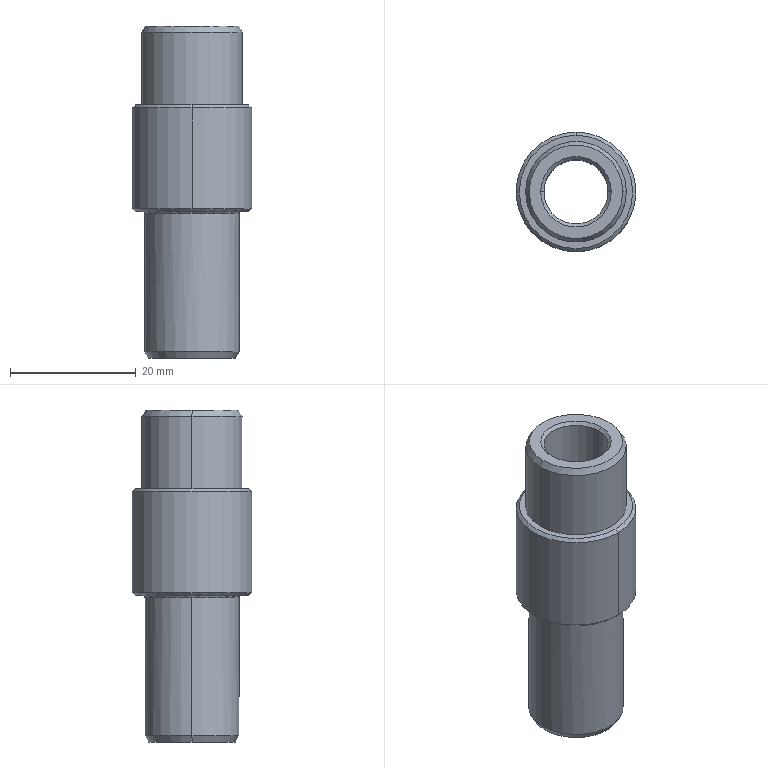Part | STEP file | PERNO RODAJA SUPERIOR | 1 solid | 26 faces | box 19 x 19 x 52.7 mm | volume 7077 mm3 | cone 12 | cylinder 8 | plane 4 | torus 2 | commonest cylinder face diameters 10.2 x2 15 x2 16 x2 19 x2
STEP:
#1=CARTESIAN_POINT('',(7.423,0.,10.5));
#2=VERTEX_POINT('',#1);
#3=CARTESIAN_POINT('',(-7.423,0.,10.5));
#4=VERTEX_POINT('',#3);
#5=CARTESIAN_POINT('',(0.,0.,10.5));
#6=DIRECTION('',(0.,0.,1.));
#7=DIRECTION('',(1.,0.,0.));
#8=AXIS2_PLACEMENT_3D('',#5,#6,#7);
#9=CIRCLE('',#8,7.423);
#10=EDGE_CURVE('',#2,#4,#9,.T.);
#11=ORIENTED_EDGE('',*,*,#10,.F.);
#12=CARTESIAN_POINT('',(8.,0.,9.5));
#13=VERTEX_POINT('',#12);
#14=CARTESIAN_POINT('',(7.423,0.,10.5));
#15=DIRECTION('',(0.5,0.,-0.866));
#16=VECTOR('',#15,1000.);
#17=LINE('',#14,#16);
#18=EDGE_CURVE('',#2,#13,#17,.T.);
#19=ORIENTED_EDGE('',*,*,#18,.T.);
#20=CARTESIAN_POINT('',(-8.,0.,9.5));
#21=VERTEX_POINT('',#20);
#22=CARTESIAN_POINT('',(0.,0.,9.5));
#23=DIRECTION('',(0.,0.,-1.));
#24=DIRECTION('',(1.,0.,0.));
#25=AXIS2_PLACEMENT_3D('',#22,#23,#24);
#26=CIRCLE('',#25,8.);
#27=EDGE_CURVE('',#21,#13,#26,.T.);
#28=ORIENTED_EDGE('',*,*,#27,.F.);
#29=CARTESIAN_POINT('',(-7.423,0.,10.5));
#30=DIRECTION('',(-0.5,0.,-0.866));
#31=VECTOR('',#30,1000.);
#32=LINE('',#29,#31);
#33=EDGE_CURVE('',#4,#21,#32,.T.);
#34=ORIENTED_EDGE('',*,*,#33,.F.);
#35=EDGE_LOOP('',(#11,#19,#28,#34));
#36=FACE_OUTER_BOUND('',#35,.T.);
#37=CARTESIAN_POINT('',(0.,0.,10.5));
#38=DIRECTION('',(0.,0.,-1.));
#39=DIRECTION('',(-1.,0.,0.));
#40=AXIS2_PLACEMENT_3D('',#37,#38,#39);
#41=CONICAL_SURFACE('',#40,7.423,0.5236);
#42=ADVANCED_FACE('',(#36),#41,.T.);
#43=CARTESIAN_POINT('',(0.,-9.,-2.));
#44=VERTEX_POINT('',#43);
#45=CARTESIAN_POINT('',(0.,9.,-2.));
#46=VERTEX_POINT('',#45);
#47=CARTESIAN_POINT('',(0.,0.,-2.));
#48=DIRECTION('',(0.,0.,1.));
#49=DIRECTION('',(0.,-1.,0.));
#50=AXIS2_PLACEMENT_3D('',#47,#48,#49);
#51=CIRCLE('',#50,9.);
#52=EDGE_CURVE('',#44,#46,#51,.T.);
#53=ORIENTED_EDGE('',*,*,#52,.F.);
#54=CARTESIAN_POINT('',(0.,-9.5,-2.5));
#55=VERTEX_POINT('',#54);
#56=CARTESIAN_POINT('',(0.,-9.5,-2.5));
#57=DIRECTION('',(0.,-0.7071,-0.7071));
#58=VECTOR('',#57,1000.);
#59=LINE('',#56,#58);
#60=EDGE_CURVE('',#44,#55,#59,.T.);
#61=ORIENTED_EDGE('',*,*,#60,.T.);
#62=CARTESIAN_POINT('',(0.,9.5,-2.5));
#63=VERTEX_POINT('',#62);
#64=CARTESIAN_POINT('',(0.,0.,-2.5));
#65=DIRECTION('',(0.,0.,-1.));
#66=DIRECTION('',(0.,-1.,0.));
#67=AXIS2_PLACEMENT_3D('',#64,#65,#66);
#68=CIRCLE('',#67,9.5);
#69=EDGE_CURVE('',#63,#55,#68,.T.);
#70=ORIENTED_EDGE('',*,*,#69,.F.);
#71=CARTESIAN_POINT('',(0.,9.5,-2.5));
#72=DIRECTION('',(0.,0.7071,-0.7071));
#73=VECTOR('',#72,1000.);
#74=LINE('',#71,#73);
#75=EDGE_CURVE('',#46,#63,#74,.T.);
#76=ORIENTED_EDGE('',*,*,#75,.F.);
#77=EDGE_LOOP('',(#53,#61,#70,#76));
#78=FACE_OUTER_BOUND('',#77,.T.);
#79=CARTESIAN_POINT('',(0.,0.,-2.5));
#80=DIRECTION('',(0.,0.,-1.));
#81=DIRECTION('',(0.,1.,0.));
#82=AXIS2_PLACEMENT_3D('',#79,#80,#81);
#83=CONICAL_SURFACE('',#82,9.5,0.7854);
#84=ADVANCED_FACE('',(#78),#83,.T.);
#85=CARTESIAN_POINT('',(0.,9.,-19.));
#86=VERTEX_POINT('',#85);
#87=CARTESIAN_POINT('',(0.,-9.,-19.));
#88=VERTEX_POINT('',#87);
#89=CARTESIAN_POINT('',(0.,0.,-19.));
#90=DIRECTION('',(0.,0.,-1.));
#91=DIRECTION('',(0.,1.,0.));
#92=AXIS2_PLACEMENT_3D('',#89,#90,#91);
#93=CIRCLE('',#92,9.);
#94=EDGE_CURVE('',#86,#88,#93,.T.);
#95=ORIENTED_EDGE('',*,*,#94,.F.);
#96=CARTESIAN_POINT('',(0.,9.5,-18.5));
#97=VERTEX_POINT('',#96);
#98=CARTESIAN_POINT('',(0.,9.,-19.));
#99=DIRECTION('',(0.,0.7071,0.7071));
#100=VECTOR('',#99,1000.);
#101=LINE('',#98,#100);
#102=EDGE_CURVE('',#86,#97,#101,.T.);
#103=ORIENTED_EDGE('',*,*,#102,.T.);
#104=CARTESIAN_POINT('',(0.,-9.5,-18.5));
#105=VERTEX_POINT('',#104);
#106=CARTESIAN_POINT('',(0.,0.,-18.5));
#107=DIRECTION('',(0.,0.,1.));
#108=DIRECTION('',(0.,1.,0.));
#109=AXIS2_PLACEMENT_3D('',#106,#107,#108);
#110=CIRCLE('',#109,9.5);
#111=EDGE_CURVE('',#105,#97,#110,.T.);
#112=ORIENTED_EDGE('',*,*,#111,.F.);
#113=CARTESIAN_POINT('',(0.,-9.,-19.));
#114=DIRECTION('',(0.,-0.7071,0.7071));
#115=VECTOR('',#114,1000.);
#116=LINE('',#113,#115);
#117=EDGE_CURVE('',#88,#105,#116,.T.);
#118=ORIENTED_EDGE('',*,*,#117,.F.);
#119=EDGE_LOOP('',(#95,#103,#112,#118));
#120=FACE_OUTER_BOUND('',#119,.T.);
#121=CARTESIAN_POINT('',(0.,0.,-19.));
#122=DIRECTION('',(0.,0.,1.));
#123=DIRECTION('',(0.,-1.,0.));
#124=AXIS2_PLACEMENT_3D('',#121,#122,#123);
#125=CONICAL_SURFACE('',#124,9.,0.7854);
#126=ADVANCED_FACE('',(#120),#125,.T.);
#127=CARTESIAN_POINT('',(-5.1,0.,10.));
#128=VERTEX_POINT('',#127);
#129=CARTESIAN_POINT('',(5.1,0.,10.));
#130=VERTEX_POINT('',#129);
#131=CARTESIAN_POINT('',(0.,0.,10.));
#132=DIRECTION('',(0.,0.,1.));
#133=DIRECTION('',(1.,0.,0.));
#134=AXIS2_PLACEMENT_3D('',#131,#132,#133);
#135=CIRCLE('',#134,5.1);
#136=EDGE_CURVE('',#128,#130,#135,.T.);
#137=ORIENTED_EDGE('',*,*,#136,.F.);
#138=CARTESIAN_POINT('',(-5.6,0.,10.5));
#139=VERTEX_POINT('',#138);
#140=CARTESIAN_POINT('',(-5.6,0.,10.5));
#141=DIRECTION('',(-0.7071,0.,0.7071));
#142=VECTOR('',#141,1000.);
#143=LINE('',#140,#142);
#144=EDGE_CURVE('',#128,#139,#143,.T.);
#145=ORIENTED_EDGE('',*,*,#144,.T.);
#146=CARTESIAN_POINT('',(5.6,0.,10.5));
#147=VERTEX_POINT('',#146);
#148=CARTESIAN_POINT('',(0.,0.,10.5));
#149=DIRECTION('',(0.,0.,-1.));
#150=DIRECTION('',(1.,0.,0.));
#151=AXIS2_PLACEMENT_3D('',#148,#149,#150);
#152=CIRCLE('',#151,5.6);
#153=EDGE_CURVE('',#147,#139,#152,.T.);
#154=ORIENTED_EDGE('',*,*,#153,.F.);
#155=CARTESIAN_POINT('',(5.6,0.,10.5));
#156=DIRECTION('',(0.7071,0.,0.7071));
#157=VECTOR('',#156,1000.);
#158=LINE('',#155,#157);
#159=EDGE_CURVE('',#130,#147,#158,.T.);
#160=ORIENTED_EDGE('',*,*,#159,.F.);
#161=EDGE_LOOP('',(#137,#145,#154,#160));
#162=FACE_OUTER_BOUND('',#161,.T.);
#163=CARTESIAN_POINT('',(0.,0.,10.5));
#164=DIRECTION('',(0.,0.,1.));
#165=DIRECTION('',(1.,0.,0.));
#166=AXIS2_PLACEMENT_3D('',#163,#164,#165);
#167=CONICAL_SURFACE('',#166,5.6,0.7854);
#168=ADVANCED_FACE('',(#162),#167,.F.);
#169=CARTESIAN_POINT('',(5.1,0.,-41.7));
#170=VERTEX_POINT('',#169);
#171=CARTESIAN_POINT('',(-5.1,0.,-41.7));
#172=VERTEX_POINT('',#171);
#173=CARTESIAN_POINT('',(0.,0.,-41.7));
#174=DIRECTION('',(0.,0.,-1.));
#175=DIRECTION('',(1.,0.,0.));
#176=AXIS2_PLACEMENT_3D('',#173,#174,#175);
#177=CIRCLE('',#176,5.1);
#178=EDGE_CURVE('',#170,#172,#177,.T.);
#179=ORIENTED_EDGE('',*,*,#178,.F.);
#180=CARTESIAN_POINT('',(5.6,0.,-42.2));
#181=VERTEX_POINT('',#180);
#182=CARTESIAN_POINT('',(5.1,0.,-41.7));
#183=DIRECTION('',(0.7071,0.,-0.7071));
#184=VECTOR('',#183,1000.);
#185=LINE('',#182,#184);
#186=EDGE_CURVE('',#170,#181,#185,.T.);
#187=ORIENTED_EDGE('',*,*,#186,.T.);
#188=CARTESIAN_POINT('',(-5.6,0.,-42.2));
#189=VERTEX_POINT('',#188);
#190=CARTESIAN_POINT('',(0.,0.,-42.2));
#191=DIRECTION('',(0.,0.,1.));
#192=DIRECTION('',(1.,0.,0.));
#193=AXIS2_PLACEMENT_3D('',#190,#191,#192);
#194=CIRCLE('',#193,5.6);
#195=EDGE_CURVE('',#189,#181,#194,.T.);
#196=ORIENTED_EDGE('',*,*,#195,.F.);
#197=CARTESIAN_POINT('',(-5.1,0.,-41.7));
#198=DIRECTION('',(-0.7071,0.,-0.7071));
#199=VECTOR('',#198,1000.);
#200=LINE('',#197,#199);
#201=EDGE_CURVE('',#172,#189,#200,.T.);
#202=ORIENTED_EDGE('',*,*,#201,.F.);
#203=EDGE_LOOP('',(#179,#187,#196,#202));
#204=FACE_OUTER_BOUND('',#203,.T.);
#205=CARTESIAN_POINT('',(0.,0.,-41.7));
#206=DIRECTION('',(0.,0.,-1.));
#207=DIRECTION('',(-1.,0.,0.));
#208=AXIS2_PLACEMENT_3D('',#205,#206,#207);
#209=CONICAL_SURFACE('',#208,5.1,0.7854);
#210=ADVANCED_FACE('',(#204),#209,.F.);
#211=ORIENTED_EDGE('',*,*,#136,.T.);
#212=CARTESIAN_POINT('',(5.1,0.,-42.2));
#213=DIRECTION('',(0.,0.,-1.));
#214=VECTOR('',#213,1000.);
#215=LINE('',#212,#214);
#216=EDGE_CURVE('',#130,#170,#215,.T.);
#217=ORIENTED_EDGE('',*,*,#216,.T.);
#218=ORIENTED_EDGE('',*,*,#178,.T.);
#219=CARTESIAN_POINT('',(-5.1,0.,-42.2));
#220=DIRECTION('',(0.,0.,-1.));
#221=VECTOR('',#220,1000.);
#222=LINE('',#219,#221);
#223=EDGE_CURVE('',#128,#172,#222,.T.);
#224=ORIENTED_EDGE('',*,*,#223,.F.);
#225=EDGE_LOOP('',(#211,#217,#218,#224));
#226=FACE_OUTER_BOUND('',#225,.T.);
#227=CARTESIAN_POINT('',(0.,0.,-42.2));
#228=DIRECTION('',(0.,0.,-1.));
#229=DIRECTION('',(-1.,0.,0.));
#230=AXIS2_PLACEMENT_3D('',#227,#228,#229);
#231=CYLINDRICAL_SURFACE('',#230,5.1);
#232=ADVANCED_FACE('',(#226),#231,.F.);
#233=CARTESIAN_POINT('',(-6.923,0.,-42.2));
#234=VERTEX_POINT('',#233);
#235=CARTESIAN_POINT('',(6.923,0.,-42.2));
#236=VERTEX_POINT('',#235);
#237=CARTESIAN_POINT('',(0.,0.,-42.2));
#238=DIRECTION('',(0.,0.,-1.));
#239=DIRECTION('',(1.,0.,0.));
#240=AXIS2_PLACEMENT_3D('',#237,#238,#239);
#241=CIRCLE('',#240,6.923);
#242=EDGE_CURVE('',#234,#236,#241,.T.);
#243=ORIENTED_EDGE('',*,*,#242,.F.);
#244=CARTESIAN_POINT('',(-7.5,0.,-41.2));
#245=VERTEX_POINT('',#244);
#246=CARTESIAN_POINT('',(-7.5,0.,-41.2));
#247=DIRECTION('',(-0.5,0.,0.866));
#248=VECTOR('',#247,1000.);
#249=LINE('',#246,#248);
#250=EDGE_CURVE('',#234,#245,#249,.T.);
#251=ORIENTED_EDGE('',*,*,#250,.T.);
#252=CARTESIAN_POINT('',(7.5,0.,-41.2));
#253=VERTEX_POINT('',#252);
#254=CARTESIAN_POINT('',(0.,0.,-41.2));
#255=DIRECTION('',(0.,0.,1.));
#256=DIRECTION('',(1.,0.,0.));
#257=AXIS2_PLACEMENT_3D('',#254,#255,#256);
#258=CIRCLE('',#257,7.5);
#259=EDGE_CURVE('',#253,#245,#258,.T.);
#260=ORIENTED_EDGE('',*,*,#259,.F.);
#261=CARTESIAN_POINT('',(7.5,0.,-41.2));
#262=DIRECTION('',(0.5,0.,0.866));
#263=VECTOR('',#262,1000.);
#264=LINE('',#261,#263);
#265=EDGE_CURVE('',#236,#253,#264,.T.);
#266=ORIENTED_EDGE('',*,*,#265,.F.);
#267=EDGE_LOOP('',(#243,#251,#260,#266));
#268=FACE_OUTER_BOUND('',#267,.T.);
#269=CARTESIAN_POINT('',(0.,0.,-41.2));
#270=DIRECTION('',(0.,0.,1.));
#271=DIRECTION('',(1.,0.,0.));
#272=AXIS2_PLACEMENT_3D('',#269,#270,#271);
#273=CONICAL_SURFACE('',#272,7.5,0.5236);
#274=ADVANCED_FACE('',(#268),#273,.T.);
#275=CARTESIAN_POINT('',(0.,-7.5,-19.2));
#276=VERTEX_POINT('',#275);
#277=CARTESIAN_POINT('',(-7.5,0.,-19.2));
#278=VERTEX_POINT('',#277);
#279=CARTESIAN_POINT('',(0.,0.,-19.2));
#280=DIRECTION('',(0.,0.,-1.));
#281=DIRECTION('',(0.,1.,0.));
#282=AXIS2_PLACEMENT_3D('',#279,#280,#281);
#283=CIRCLE('',#282,7.5);
#284=EDGE_CURVE('',#276,#278,#283,.T.);
#285=ORIENTED_EDGE('',*,*,#284,.F.);
#286=CARTESIAN_POINT('',(0.,-7.7,-19.));
#287=VERTEX_POINT('',#286);
#288=CARTESIAN_POINT('',(0.,-7.7,-19.2));
#289=DIRECTION('',(1.,0.,0.));
#290=DIRECTION('',(0.,1.,0.));
#291=AXIS2_PLACEMENT_3D('',#288,#289,#290);
#292=CIRCLE('',#291,0.2);
#293=EDGE_CURVE('',#276,#287,#292,.T.);
#294=ORIENTED_EDGE('',*,*,#293,.T.);
#295=CARTESIAN_POINT('',(0.,7.7,-19.));
#296=VERTEX_POINT('',#295);
#297=CARTESIAN_POINT('',(0.,0.,-19.));
#298=DIRECTION('',(0.,0.,1.));
#299=DIRECTION('',(0.,1.,0.));
#300=AXIS2_PLACEMENT_3D('',#297,#298,#299);
#301=CIRCLE('',#300,7.7);
#302=EDGE_CURVE('',#296,#287,#301,.T.);
#303=ORIENTED_EDGE('',*,*,#302,.F.);
#304=CARTESIAN_POINT('',(0.,7.5,-19.2));
#305=VERTEX_POINT('',#304);
#306=CARTESIAN_POINT('',(0.,7.7,-19.2));
#307=DIRECTION('',(-1.,0.,0.));
#308=DIRECTION('',(0.,0.,1.));
#309=AXIS2_PLACEMENT_3D('',#306,#307,#308);
#310=CIRCLE('',#309,0.2);
#311=EDGE_CURVE('',#305,#296,#310,.T.);
#312=ORIENTED_EDGE('',*,*,#311,.F.);
#313=CARTESIAN_POINT('',(0.,0.,-19.2));
#314=DIRECTION('',(0.,0.,-1.));
#315=DIRECTION('',(0.,1.,0.));
#316=AXIS2_PLACEMENT_3D('',#313,#314,#315);
#317=CIRCLE('',#316,7.5);
#318=EDGE_CURVE('',#278,#305,#317,.T.);
#319=ORIENTED_EDGE('',*,*,#318,.F.);
#320=EDGE_LOOP('',(#285,#294,#303,#312,#319));
#321=FACE_OUTER_BOUND('',#320,.T.);
#322=CARTESIAN_POINT('',(0.,0.,-19.2));
#323=DIRECTION('',(0.,0.,-1.));
#324=DIRECTION('',(0.,1.,0.));
#325=AXIS2_PLACEMENT_3D('',#322,#323,#324);
#326=TOROIDAL_SURFACE('',#325,7.7,0.2);
#327=ADVANCED_FACE('',(#321),#326,.F.);
#328=ORIENTED_EDGE('',*,*,#259,.T.);
#329=CARTESIAN_POINT('',(-7.5,0.,-42.2));
#330=DIRECTION('',(0.,0.,1.));
#331=VECTOR('',#330,1000.);
#332=LINE('',#329,#331);
#333=EDGE_CURVE('',#245,#278,#332,.T.);
#334=ORIENTED_EDGE('',*,*,#333,.T.);
#335=ORIENTED_EDGE('',*,*,#318,.T.);
#336=CARTESIAN_POINT('',(7.5,0.,-19.2));
#337=VERTEX_POINT('',#336);
#338=CARTESIAN_POINT('',(0.,0.,-19.2));
#339=DIRECTION('',(0.,0.,-1.));
#340=DIRECTION('',(0.,1.,0.));
#341=AXIS2_PLACEMENT_3D('',#338,#339,#340);
#342=CIRCLE('',#341,7.5);
#343=EDGE_CURVE('',#305,#337,#342,.T.);
#344=ORIENTED_EDGE('',*,*,#343,.T.);
#345=CARTESIAN_POINT('',(7.5,0.,-42.2));
#346=DIRECTION('',(0.,0.,1.));
#347=VECTOR('',#346,1000.);
#348=LINE('',#345,#347);
#349=EDGE_CURVE('',#253,#337,#348,.T.);
#350=ORIENTED_EDGE('',*,*,#349,.F.);
#351=EDGE_LOOP('',(#328,#334,#335,#344,#350));
#352=FACE_OUTER_BOUND('',#351,.T.);
#353=CARTESIAN_POINT('',(0.,0.,-42.2));
#354=DIRECTION('',(0.,0.,1.));
#355=DIRECTION('',(1.,0.,0.));
#356=AXIS2_PLACEMENT_3D('',#353,#354,#355);
#357=CYLINDRICAL_SURFACE('',#356,7.5);
#358=ADVANCED_FACE('',(#352),#357,.T.);
#359=ORIENTED_EDGE('',*,*,#69,.T.);
#360=CARTESIAN_POINT('',(0.,-9.5,-19.));
#361=DIRECTION('',(0.,0.,-1.));
#362=VECTOR('',#361,1000.);
#363=LINE('',#360,#362);
#364=EDGE_CURVE('',#55,#105,#363,.T.);
#365=ORIENTED_EDGE('',*,*,#364,.T.);
#366=ORIENTED_EDGE('',*,*,#111,.T.);
#367=CARTESIAN_POINT('',(0.,9.5,-19.));
#368=DIRECTION('',(0.,0.,-1.));
#369=VECTOR('',#368,1000.);
#370=LINE('',#367,#369);
#371=EDGE_CURVE('',#63,#97,#370,.T.);
#372=ORIENTED_EDGE('',*,*,#371,.F.);
#373=EDGE_LOOP('',(#359,#365,#366,#372));
#374=FACE_OUTER_BOUND('',#373,.T.);
#375=CARTESIAN_POINT('',(0.,0.,-19.));
#376=DIRECTION('',(0.,0.,-1.));
#377=DIRECTION('',(0.,1.,0.));
#378=AXIS2_PLACEMENT_3D('',#375,#376,#377);
#379=CYLINDRICAL_SURFACE('',#378,9.5);
#380=ADVANCED_FACE('',(#374),#379,.T.);
#381=CARTESIAN_POINT('',(-8.,0.,-2.));
#382=VERTEX_POINT('',#381);
#383=CARTESIAN_POINT('',(8.,0.,-2.));
#384=VERTEX_POINT('',#383);
#385=CARTESIAN_POINT('',(0.,0.,-2.));
#386=DIRECTION('',(0.,0.,-1.));
#387=DIRECTION('',(0.,-1.,0.));
#388=AXIS2_PLACEMENT_3D('',#385,#386,#387);
#389=CIRCLE('',#388,8.);
#390=EDGE_CURVE('',#382,#384,#389,.T.);
#391=ORIENTED_EDGE('',*,*,#390,.F.);
#392=CARTESIAN_POINT('',(-8.,0.,-42.2));
#393=DIRECTION('',(0.,0.,1.));
#394=VECTOR('',#393,1000.);
#395=LINE('',#392,#394);
#396=EDGE_CURVE('',#382,#21,#395,.T.);
#397=ORIENTED_EDGE('',*,*,#396,.T.);
#398=ORIENTED_EDGE('',*,*,#27,.T.);
#399=CARTESIAN_POINT('',(8.,0.,-42.2));
#400=DIRECTION('',(0.,0.,1.));
#401=VECTOR('',#400,1000.);
#402=LINE('',#399,#401);
#403=EDGE_CURVE('',#384,#13,#402,.T.);
#404=ORIENTED_EDGE('',*,*,#403,.F.);
#405=EDGE_LOOP('',(#391,#397,#398,#404));
#406=FACE_OUTER_BOUND('',#405,.T.);
#407=CARTESIAN_POINT('',(0.,0.,-42.2));
#408=DIRECTION('',(0.,0.,1.));
#409=DIRECTION('',(1.,0.,0.));
#410=AXIS2_PLACEMENT_3D('',#407,#408,#409);
#411=CYLINDRICAL_SURFACE('',#410,8.);
#412=ADVANCED_FACE('',(#406),#411,.T.);
#413=ORIENTED_EDGE('',*,*,#396,.F.);
#414=CARTESIAN_POINT('',(0.,0.,-2.));
#415=DIRECTION('',(0.,0.,-1.));
#416=DIRECTION('',(0.,-1.,0.));
#417=AXIS2_PLACEMENT_3D('',#414,#415,#416);
#418=CIRCLE('',#417,8.);
#419=EDGE_CURVE('',#384,#382,#418,.T.);
#420=ORIENTED_EDGE('',*,*,#419,.F.);
#421=ORIENTED_EDGE('',*,*,#403,.T.);
#422=CARTESIAN_POINT('',(0.,0.,9.5));
#423=DIRECTION('',(0.,0.,-1.));
#424=DIRECTION('',(1.,0.,0.));
#425=AXIS2_PLACEMENT_3D('',#422,#423,#424);
#426=CIRCLE('',#425,8.);
#427=EDGE_CURVE('',#13,#21,#426,.T.);
#428=ORIENTED_EDGE('',*,*,#427,.T.);
#429=EDGE_LOOP('',(#413,#420,#421,#428));
#430=FACE_OUTER_BOUND('',#429,.T.);
#431=CARTESIAN_POINT('',(0.,0.,-42.2));
#432=DIRECTION('',(0.,0.,1.));
#433=DIRECTION('',(1.,0.,0.));
#434=AXIS2_PLACEMENT_3D('',#431,#432,#433);
#435=CYLINDRICAL_SURFACE('',#434,8.);
#436=ADVANCED_FACE('',(#430),#435,.T.);
#437=CARTESIAN_POINT('',(0.,0.,10.5));
#438=DIRECTION('',(0.,0.,1.));
#439=DIRECTION('',(1.,0.,0.));
#440=AXIS2_PLACEMENT_3D('',#437,#438,#439);
#441=CIRCLE('',#440,7.423);
#442=EDGE_CURVE('',#4,#2,#441,.T.);
#443=ORIENTED_EDGE('',*,*,#442,.T.);
#444=ORIENTED_EDGE('',*,*,#10,.T.);
#445=EDGE_LOOP('',(#443,#444));
#446=FACE_OUTER_BOUND('',#445,.T.);
#447=ORIENTED_EDGE('',*,*,#153,.T.);
#448=CARTESIAN_POINT('',(0.,0.,10.5));
#449=DIRECTION('',(0.,0.,-1.));
#450=DIRECTION('',(1.,0.,0.));
#451=AXIS2_PLACEMENT_3D('',#448,#449,#450);
#452=CIRCLE('',#451,5.6);
#453=EDGE_CURVE('',#139,#147,#452,.T.);
#454=ORIENTED_EDGE('',*,*,#453,.T.);
#455=EDGE_LOOP('',(#447,#454));
#456=FACE_BOUND('',#455,.T.);
#457=CARTESIAN_POINT('',(0.,0.,10.5));
#458=DIRECTION('',(0.,0.,1.));
#459=DIRECTION('',(1.,0.,0.));
#460=AXIS2_PLACEMENT_3D('',#457,#458,#459);
#461=PLANE('',#460);
#462=ADVANCED_FACE('',(#446,#456),#461,.T.);
#463=CARTESIAN_POINT('',(0.,0.,-2.));
#464=DIRECTION('',(0.,0.,1.));
#465=DIRECTION('',(0.,-1.,0.));
#466=AXIS2_PLACEMENT_3D('',#463,#464,#465);
#467=CIRCLE('',#466,9.);
#468=EDGE_CURVE('',#46,#44,#467,.T.);
#469=ORIENTED_EDGE('',*,*,#468,.T.);
#470=ORIENTED_EDGE('',*,*,#52,.T.);
#471=EDGE_LOOP('',(#469,#470));
#472=FACE_OUTER_BOUND('',#471,.T.);
#473=ORIENTED_EDGE('',*,*,#419,.T.);
#474=ORIENTED_EDGE('',*,*,#390,.T.);
#475=EDGE_LOOP('',(#473,#474));
#476=FACE_BOUND('',#475,.T.);
#477=CARTESIAN_POINT('',(0.,0.,-2.));
#478=DIRECTION('',(0.,0.,1.));
#479=DIRECTION('',(0.,-1.,0.));
#480=AXIS2_PLACEMENT_3D('',#477,#478,#479);
#481=PLANE('',#480);
#482=ADVANCED_FACE('',(#472,#476),#481,.T.);
#483=ORIENTED_EDGE('',*,*,#364,.F.);
#484=CARTESIAN_POINT('',(0.,0.,-2.5));
#485=DIRECTION('',(0.,0.,-1.));
#486=DIRECTION('',(0.,-1.,0.));
#487=AXIS2_PLACEMENT_3D('',#484,#485,#486);
#488=CIRCLE('',#487,9.5);
#489=EDGE_CURVE('',#55,#63,#488,.T.);
#490=ORIENTED_EDGE('',*,*,#489,.T.);
#491=ORIENTED_EDGE('',*,*,#371,.T.);
#492=CARTESIAN_POINT('',(0.,0.,-18.5));
#493=DIRECTION('',(0.,0.,1.));
#494=DIRECTION('',(0.,1.,0.));
#495=AXIS2_PLACEMENT_3D('',#492,#493,#494);
#496=CIRCLE('',#495,9.5);
#497=EDGE_CURVE('',#97,#105,#496,.T.);
#498=ORIENTED_EDGE('',*,*,#497,.T.);
#499=EDGE_LOOP('',(#483,#490,#491,#498));
#500=FACE_OUTER_BOUND('',#499,.T.);
#501=CARTESIAN_POINT('',(0.,0.,-19.));
#502=DIRECTION('',(0.,0.,-1.));
#503=DIRECTION('',(0.,1.,0.));
#504=AXIS2_PLACEMENT_3D('',#501,#502,#503);
#505=CYLINDRICAL_SURFACE('',#504,9.5);
#506=ADVANCED_FACE('',(#500),#505,.T.);
#507=CARTESIAN_POINT('',(0.,0.,-19.));
#508=DIRECTION('',(0.,0.,-1.));
#509=DIRECTION('',(0.,1.,0.));
#510=AXIS2_PLACEMENT_3D('',#507,#508,#509);
#511=CIRCLE('',#510,9.);
#512=EDGE_CURVE('',#88,#86,#511,.T.);
#513=ORIENTED_EDGE('',*,*,#512,.T.);
#514=ORIENTED_EDGE('',*,*,#94,.T.);
#515=EDGE_LOOP('',(#513,#514));
#516=FACE_OUTER_BOUND('',#515,.T.);
#517=ORIENTED_EDGE('',*,*,#302,.T.);
#518=CARTESIAN_POINT('',(0.,0.,-19.));
#519=DIRECTION('',(0.,0.,1.));
#520=DIRECTION('',(0.,1.,0.));
#521=AXIS2_PLACEMENT_3D('',#518,#519,#520);
#522=CIRCLE('',#521,7.7);
#523=EDGE_CURVE('',#287,#296,#522,.T.);
#524=ORIENTED_EDGE('',*,*,#523,.T.);
#525=EDGE_LOOP('',(#517,#524));
#526=FACE_BOUND('',#525,.T.);
#527=CARTESIAN_POINT('',(0.,9.5,-19.));
#528=DIRECTION('',(0.,0.,-1.));
#529=DIRECTION('',(0.,1.,0.));
#530=AXIS2_PLACEMENT_3D('',#527,#528,#529);
#531=PLANE('',#530);
#532=ADVANCED_FACE('',(#516,#526),#531,.T.);
#533=ORIENTED_EDGE('',*,*,#195,.T.);
#534=CARTESIAN_POINT('',(0.,0.,-42.2));
#535=DIRECTION('',(0.,0.,1.));
#536=DIRECTION('',(1.,0.,0.));
#537=AXIS2_PLACEMENT_3D('',#534,#535,#536);
#538=CIRCLE('',#537,5.6);
#539=EDGE_CURVE('',#181,#189,#538,.T.);
#540=ORIENTED_EDGE('',*,*,#539,.T.);
#541=EDGE_LOOP('',(#533,#540));
#542=FACE_BOUND('',#541,.T.);
#543=CARTESIAN_POINT('',(0.,0.,-42.2));
#544=DIRECTION('',(0.,0.,-1.));
#545=DIRECTION('',(1.,0.,0.));
#546=AXIS2_PLACEMENT_3D('',#543,#544,#545);
#547=CIRCLE('',#546,6.923);
#548=EDGE_CURVE('',#236,#234,#547,.T.);
#549=ORIENTED_EDGE('',*,*,#548,.T.);
#550=ORIENTED_EDGE('',*,*,#242,.T.);
#551=EDGE_LOOP('',(#549,#550));
#552=FACE_OUTER_BOUND('',#551,.T.);
#553=CARTESIAN_POINT('',(0.,0.,-42.2));
#554=DIRECTION('',(0.,0.,1.));
#555=DIRECTION('',(1.,0.,0.));
#556=AXIS2_PLACEMENT_3D('',#553,#554,#555);
#557=PLANE('',#556);
#558=ADVANCED_FACE('',(#542,#552),#557,.F.);
#559=ORIENTED_EDGE('',*,*,#333,.F.);
#560=CARTESIAN_POINT('',(0.,0.,-41.2));
#561=DIRECTION('',(0.,0.,1.));
#562=DIRECTION('',(1.,0.,0.));
#563=AXIS2_PLACEMENT_3D('',#560,#561,#562);
#564=CIRCLE('',#563,7.5);
#565=EDGE_CURVE('',#245,#253,#564,.T.);
#566=ORIENTED_EDGE('',*,*,#565,.T.);
#567=ORIENTED_EDGE('',*,*,#349,.T.);
#568=CARTESIAN_POINT('',(0.,0.,-19.2));
#569=DIRECTION('',(0.,0.,-1.));
#570=DIRECTION('',(0.,1.,0.));
#571=AXIS2_PLACEMENT_3D('',#568,#569,#570);
#572=CIRCLE('',#571,7.5);
#573=EDGE_CURVE('',#337,#276,#572,.T.);
#574=ORIENTED_EDGE('',*,*,#573,.T.);
#575=ORIENTED_EDGE('',*,*,#284,.T.);
#576=EDGE_LOOP('',(#559,#566,#567,#574,#575));
#577=FACE_OUTER_BOUND('',#576,.T.);
#578=CARTESIAN_POINT('',(0.,0.,-42.2));
#579=DIRECTION('',(0.,0.,1.));
#580=DIRECTION('',(1.,0.,0.));
#581=AXIS2_PLACEMENT_3D('',#578,#579,#580);
#582=CYLINDRICAL_SURFACE('',#581,7.5);
#583=ADVANCED_FACE('',(#577),#582,.T.);
#584=ORIENTED_EDGE('',*,*,#293,.F.);
#585=ORIENTED_EDGE('',*,*,#573,.F.);
#586=ORIENTED_EDGE('',*,*,#343,.F.);
#587=ORIENTED_EDGE('',*,*,#311,.T.);
#588=ORIENTED_EDGE('',*,*,#523,.F.);
#589=EDGE_LOOP('',(#584,#585,#586,#587,#588));
#590=FACE_OUTER_BOUND('',#589,.T.);
#591=CARTESIAN_POINT('',(0.,0.,-19.2));
#592=DIRECTION('',(0.,0.,-1.));
#593=DIRECTION('',(0.,1.,0.));
#594=AXIS2_PLACEMENT_3D('',#591,#592,#593);
#595=TOROIDAL_SURFACE('',#594,7.7,0.2);
#596=ADVANCED_FACE('',(#590),#595,.F.);
#597=ORIENTED_EDGE('',*,*,#250,.F.);
#598=ORIENTED_EDGE('',*,*,#548,.F.);
#599=ORIENTED_EDGE('',*,*,#265,.T.);
#600=ORIENTED_EDGE('',*,*,#565,.F.);
#601=EDGE_LOOP('',(#597,#598,#599,#600));
#602=FACE_OUTER_BOUND('',#601,.T.);
#603=CARTESIAN_POINT('',(0.,0.,-41.2));
#604=DIRECTION('',(0.,0.,1.));
#605=DIRECTION('',(1.,0.,0.));
#606=AXIS2_PLACEMENT_3D('',#603,#604,#605);
#607=CONICAL_SURFACE('',#606,7.5,0.5236);
#608=ADVANCED_FACE('',(#602),#607,.T.);
#609=ORIENTED_EDGE('',*,*,#216,.F.);
#610=CARTESIAN_POINT('',(0.,0.,10.));
#611=DIRECTION('',(0.,0.,1.));
#612=DIRECTION('',(1.,0.,0.));
#613=AXIS2_PLACEMENT_3D('',#610,#611,#612);
#614=CIRCLE('',#613,5.1);
#615=EDGE_CURVE('',#130,#128,#614,.T.);
#616=ORIENTED_EDGE('',*,*,#615,.T.);
#617=ORIENTED_EDGE('',*,*,#223,.T.);
#618=CARTESIAN_POINT('',(0.,0.,-41.7));
#619=DIRECTION('',(0.,0.,-1.));
#620=DIRECTION('',(1.,0.,0.));
#621=AXIS2_PLACEMENT_3D('',#618,#619,#620);
#622=CIRCLE('',#621,5.1);
#623=EDGE_CURVE('',#172,#170,#622,.T.);
#624=ORIENTED_EDGE('',*,*,#623,.T.);
#625=EDGE_LOOP('',(#609,#616,#617,#624));
#626=FACE_OUTER_BOUND('',#625,.T.);
#627=CARTESIAN_POINT('',(0.,0.,-42.2));
#628=DIRECTION('',(0.,0.,-1.));
#629=DIRECTION('',(-1.,0.,0.));
#630=AXIS2_PLACEMENT_3D('',#627,#628,#629);
#631=CYLINDRICAL_SURFACE('',#630,5.1);
#632=ADVANCED_FACE('',(#626),#631,.F.);
#633=ORIENTED_EDGE('',*,*,#186,.F.);
#634=ORIENTED_EDGE('',*,*,#623,.F.);
#635=ORIENTED_EDGE('',*,*,#201,.T.);
#636=ORIENTED_EDGE('',*,*,#539,.F.);
#637=EDGE_LOOP('',(#633,#634,#635,#636));
#638=FACE_OUTER_BOUND('',#637,.T.);
#639=CARTESIAN_POINT('',(0.,0.,-41.7));
#640=DIRECTION('',(0.,0.,-1.));
#641=DIRECTION('',(-1.,0.,0.));
#642=AXIS2_PLACEMENT_3D('',#639,#640,#641);
#643=CONICAL_SURFACE('',#642,5.1,0.7854);
#644=ADVANCED_FACE('',(#638),#643,.F.);
#645=ORIENTED_EDGE('',*,*,#144,.F.);
#646=ORIENTED_EDGE('',*,*,#615,.F.);
#647=ORIENTED_EDGE('',*,*,#159,.T.);
#648=ORIENTED_EDGE('',*,*,#453,.F.);
#649=EDGE_LOOP('',(#645,#646,#647,#648));
#650=FACE_OUTER_BOUND('',#649,.T.);
#651=CARTESIAN_POINT('',(0.,0.,10.5));
#652=DIRECTION('',(0.,0.,1.));
#653=DIRECTION('',(1.,0.,0.));
#654=AXIS2_PLACEMENT_3D('',#651,#652,#653);
#655=CONICAL_SURFACE('',#654,5.6,0.7854);
#656=ADVANCED_FACE('',(#650),#655,.F.);
#657=ORIENTED_EDGE('',*,*,#102,.F.);
#658=ORIENTED_EDGE('',*,*,#512,.F.);
#659=ORIENTED_EDGE('',*,*,#117,.T.);
#660=ORIENTED_EDGE('',*,*,#497,.F.);
#661=EDGE_LOOP('',(#657,#658,#659,#660));
#662=FACE_OUTER_BOUND('',#661,.T.);
#663=CARTESIAN_POINT('',(0.,0.,-19.));
#664=DIRECTION('',(0.,0.,1.));
#665=DIRECTION('',(0.,-1.,0.));
#666=AXIS2_PLACEMENT_3D('',#663,#664,#665);
#667=CONICAL_SURFACE('',#666,9.,0.7854);
#668=ADVANCED_FACE('',(#662),#667,.T.);
#669=ORIENTED_EDGE('',*,*,#60,.F.);
#670=ORIENTED_EDGE('',*,*,#468,.F.);
#671=ORIENTED_EDGE('',*,*,#75,.T.);
#672=ORIENTED_EDGE('',*,*,#489,.F.);
#673=EDGE_LOOP('',(#669,#670,#671,#672));
#674=FACE_OUTER_BOUND('',#673,.T.);
#675=CARTESIAN_POINT('',(0.,0.,-2.5));
#676=DIRECTION('',(0.,0.,-1.));
#677=DIRECTION('',(0.,1.,0.));
#678=AXIS2_PLACEMENT_3D('',#675,#676,#677);
#679=CONICAL_SURFACE('',#678,9.5,0.7854);
#680=ADVANCED_FACE('',(#674),#679,.T.);
#681=ORIENTED_EDGE('',*,*,#18,.F.);
#682=ORIENTED_EDGE('',*,*,#442,.F.);
#683=ORIENTED_EDGE('',*,*,#33,.T.);
#684=ORIENTED_EDGE('',*,*,#427,.F.);
#685=EDGE_LOOP('',(#681,#682,#683,#684));
#686=FACE_OUTER_BOUND('',#685,.T.);
#687=CARTESIAN_POINT('',(0.,0.,10.5));
#688=DIRECTION('',(0.,0.,-1.));
#689=DIRECTION('',(-1.,0.,0.));
#690=AXIS2_PLACEMENT_3D('',#687,#688,#689);
#691=CONICAL_SURFACE('',#690,7.423,0.5236);
#692=ADVANCED_FACE('',(#686),#691,.T.);
#693=CLOSED_SHELL('',(#42,#84,#126,#168,#210,#232,#274,#327,#358,#380,#412,#436,#462,#482,#506,#532,#558,#583,#596,#608,#632,#644,#656,#668,#680,#692));
#694=MANIFOLD_SOLID_BREP('',#693);
#695=CARTESIAN_POINT('',(0.,0.,0.));
#696=DIRECTION('',(0.,0.,1.));
#697=DIRECTION('',(1.,0.,0.));
#698=AXIS2_PLACEMENT_3D('',#695,#696,#697);
#699=(LENGTH_UNIT()NAMED_UNIT(*)SI_UNIT(.MILLI.,.METRE.));
#700=UNCERTAINTY_MEASURE_WITH_UNIT(LENGTH_MEASURE(0.00001),#699,'','');
#701=(NAMED_UNIT(*)PLANE_ANGLE_UNIT()SI_UNIT($,.RADIAN.));
#702=(NAMED_UNIT(*)SI_UNIT($,.STERADIAN.)SOLID_ANGLE_UNIT());
#703=(GEOMETRIC_REPRESENTATION_CONTEXT(3)GLOBAL_UNCERTAINTY_ASSIGNED_CONTEXT((#700))GLOBAL_UNIT_ASSIGNED_CONTEXT((#699,#701,#702))REPRESENTATION_CONTEXT('',''));
#704=ADVANCED_BREP_SHAPE_REPRESENTATION('',(#694,#698),#703);